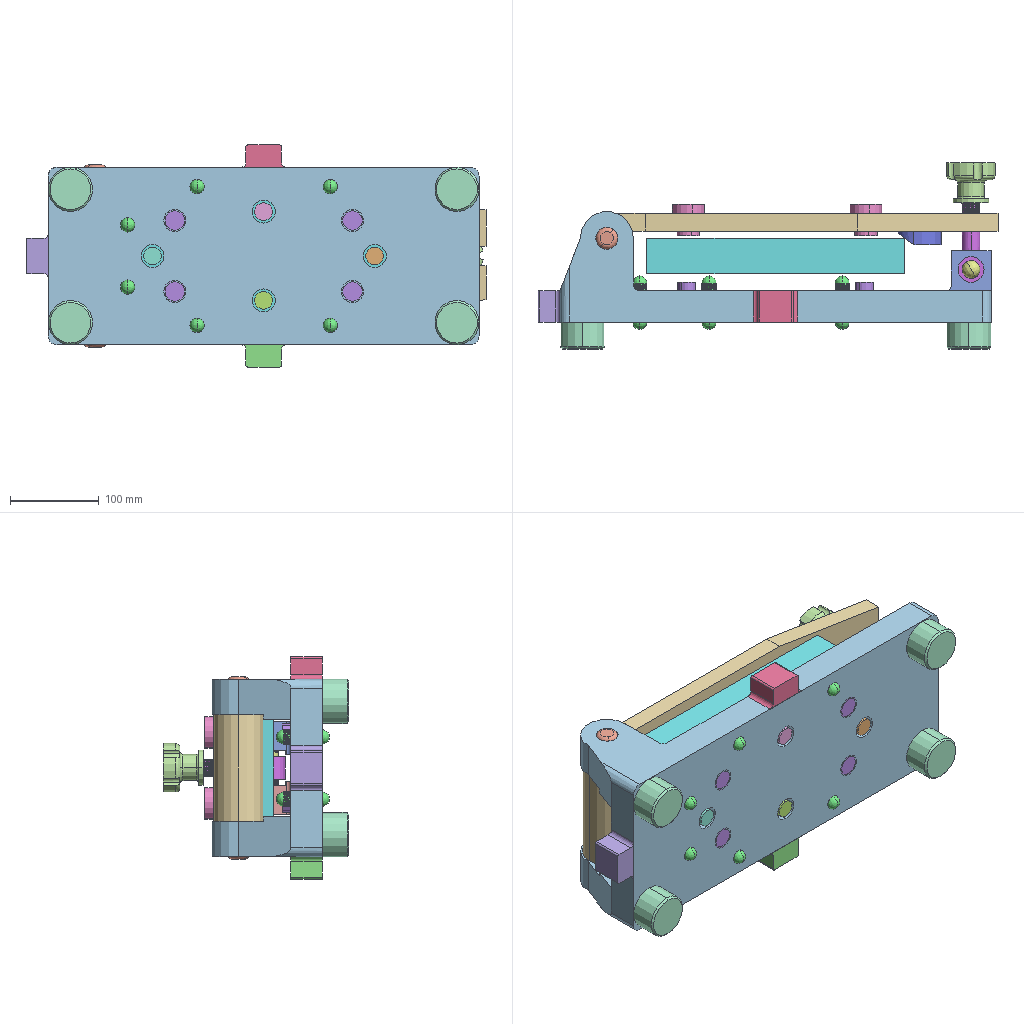Assembly | SolidWorks | 13 different items | 27 placed | box 518 x 209 x 250 mm
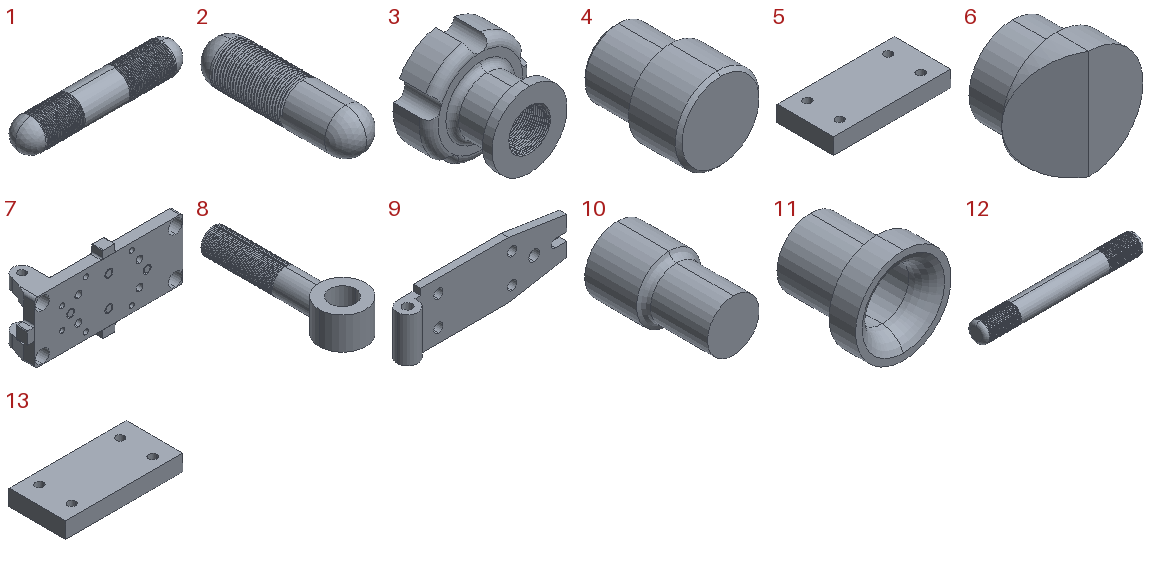Parts list (item | quantity | size | volume | features):
1 | x1 | 105 x 20 x 20 mm | 30081 mm3 | features SweepThread 2, Fillet 1, RevolutionThin 1
2 | x6 | 16 x 60 x 16 mm | 10676 mm3 | features Fillet 2, Revolution 1, SweepThread 1
3 | x1 | 55 x 45.25 x 54.545 mm | 45993 mm3 | features ICE 1, Revolution 1, SweepThread 1
4 | x4 | 50 x 63 x 50 mm | 98942 mm3 | features Chamfer 2, Revolution 1
5 | x1 | 290 x 140 x 40 mm | 1573735 mm3 | features Extrusion 1
6 | x1 | 50 x 35 x 50 mm | 47619 mm3 | features ICE 1, Revolution 1
7 | x1 | 510.004 x 124.441 x 250 mm | 3715115 mm3 | features ICE 6, Extrusion 1, Fillet 1
8 | x1 | 36 x 118 x 25 mm | 42808 mm3 | features Extrusion 1, Revolution 1, SweepThread 1
9 | x1 | 468.278 x 56 x 153.374 mm | 1357843 mm3 | features Extrusion 1, ICE 1
10 | x4 | 25 x 45 x 25 mm | 17793 mm3 | features Fillet 1, Revolution 1
11 | x4 | 35.913 x 35 x 35.913 mm | 10695 mm3 | features Revolution 1
12 | x1 | 205 x 25 x 25 mm | 98310 mm3 | features SweepThread 2, Fillet 1, Revolution 1
13 | x1 | 290 x 140 x 40 mm | 1573735 mm3 | features Extrusion 1
Mates (type | each side: item.copy, entity, surface, feature):
Coincident | 7.1 plane | assembly plane | 3 times
Concentric | 7.1 face cylinder Boss-Extrude2 | 1.1 face cylinder Revolve-Thin1
Tangent | 7.1 face plane Boss-Extrude2 | 1.1 face sphere Fillet1
Concentric | 1.1 face cylinder Revolve-Thin1 | 8.1 face cylinder Boss-Extrude1
Concentric | 7.1 face cylinder Cut-Extrude5 | 4.1 face cylinder Revolve1
Coincident | 7.1 face plane Boss-Extrude1 | 4.1 face plane Revolve1
Coincident | 7.1 face plane Boss-Extrude1 | 4.2 face plane Revolve1
Concentric | 7.1 face cylinder Boss-Extrude1 | 12.1 face cylinder Revolve2
DistanceDim | 12.1 face plane Revolve2 | 7.1 face plane Boss-Extrude1
Concentric | 7.1 face cylinder Cut-Extrude4 | 13.1 face cylinder Boss-Extrude1 | 2 times
Width | 7.1 face plane Cut-Extrude1 | 7.1 face plane Cut-Extrude1 | 9.1 face plane Boss-Extrude1 | 9.1 face plane Boss-Extrude1
Concentric | 12.1 face cylinder Revolve2 | 9.1 face cylinder Boss-Extrude3
Width | 9.1 face plane Boss-Extrude1 | 9.1 face plane Boss-Extrude1 | 8.1 face cylinder Revolve1
Concentric | 6.1 face cylinder Revolve2 | 9.1 face cylinder Boss-Extrude1
Coincident | 6.1 edge | 9.1 face plane Boss-Extrude1
Tangent | 8.1 edge | 3.1 edge
Parallel | 3.1 face plane Revolve1 | 9.1 face plane Boss-Extrude1
Concentric | 11.1 face cylinder Revolve2 | 9.1 face cylinder Boss-Extrude1
Concentric | 11.2 face cylinder Revolve2 | 9.1 face cylinder Boss-Extrude1
Concentric | 11.3 face cylinder Revolve2 | 9.1 face cylinder Boss-Extrude1
Concentric | 11.4 face cylinder Revolve2 | 9.1 face cylinder Boss-Extrude1
Coincident | 11.2 face plane Revolve2 | 9.1 face plane Boss-Extrude1
Coincident | 11.1 face plane Revolve2 | 9.1 face plane Boss-Extrude1
Coincident | 11.3 face plane Revolve2 | 9.1 face plane Boss-Extrude1
Coincident | 11.4 face plane Revolve2 | 9.1 face plane Boss-Extrude1
Concentric | 7.1 face cylinder Cut-Extrude4 | 10.1 face cylinder Revolve1
Concentric | 7.1 face cylinder Cut-Extrude4 | 10.2 face cylinder Revolve1
Concentric | 7.1 face cylinder Cut-Extrude4 | 10.3 face cylinder Revolve1
Concentric | 7.1 face cylinder Cut-Extrude4 | 10.4 face cylinder Revolve1
DistanceDim | 13.1 face plane Boss-Extrude1 | 9.1 face plane Boss-Extrude1
Coincident | 7.1 face plane Boss-Extrude1 | 10.4 face plane Revolve1
Coincident | 7.1 face plane Boss-Extrude1 | 10.1 face plane Revolve1
Coincident | 7.1 face plane Boss-Extrude1 | 10.2 face plane Revolve1
Coincident | 7.1 face plane Boss-Extrude1 | 10.3 face plane Revolve1
Concentric | 7.1 face cylinder Cut-Extrude4 | 2.1 face cylinder Revolve1
Coincident | 7.1 face plane Boss-Extrude1 | 2.1 edge
Coincident | 7.1 face plane Boss-Extrude1 | 2.2 edge
Concentric | 7.1 face cylinder Cut-Extrude4 | 2.3 face cylinder Revolve1
Coincident | 7.1 face plane Boss-Extrude1 | 2.3 edge
Concentric | 7.1 face cylinder Cut-Extrude4 | 2.4 face cylinder Revolve1
Coincident | 7.1 face plane Boss-Extrude1 | 2.4 edge
Concentric | 7.1 face cylinder Cut-Extrude4 | 2.5 face cylinder Revolve1
Coincident | 7.1 face plane Boss-Extrude1 | 2.5 edge
Concentric | 7.1 face cylinder Cut-Extrude4 | 2.6 face cylinder Revolve1
Coincident | 7.1 face plane Boss-Extrude1 | 2.6 edge
Concentric | 4.3 face cylinder Revolve1 | 7.1 face cylinder Cut-Extrude5
Coincident | 7.1 face plane Boss-Extrude1 | 4.3 face plane Revolve1
Concentric | 7.1 face cylinder Cut-Extrude5 | 4.4 face cylinder Revolve1
Coincident | 7.1 face plane Boss-Extrude1 | 4.4 face plane Revolve1